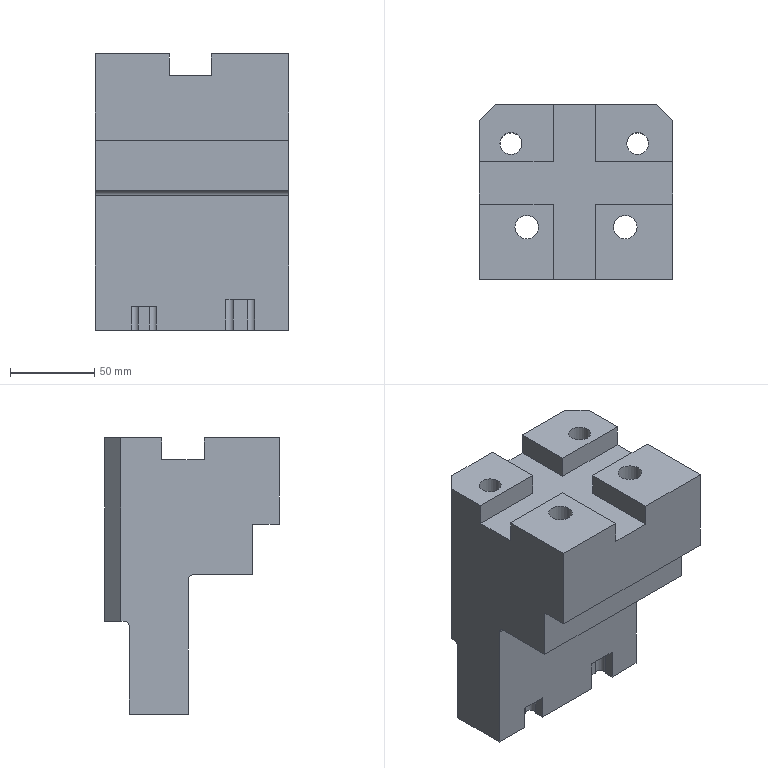Part | STEP file | 1_id154_x_t | 1 solid | 81 faces | box 114.3 x 103.32 x 163.553 mm | volume 1067173 mm3 | plane 50 | cylinder 26 | cone 5 | commonest cylinder face diameters 6 x10 6.75 x4 20 x4 3.3 x2 6.8 x2 13 x2